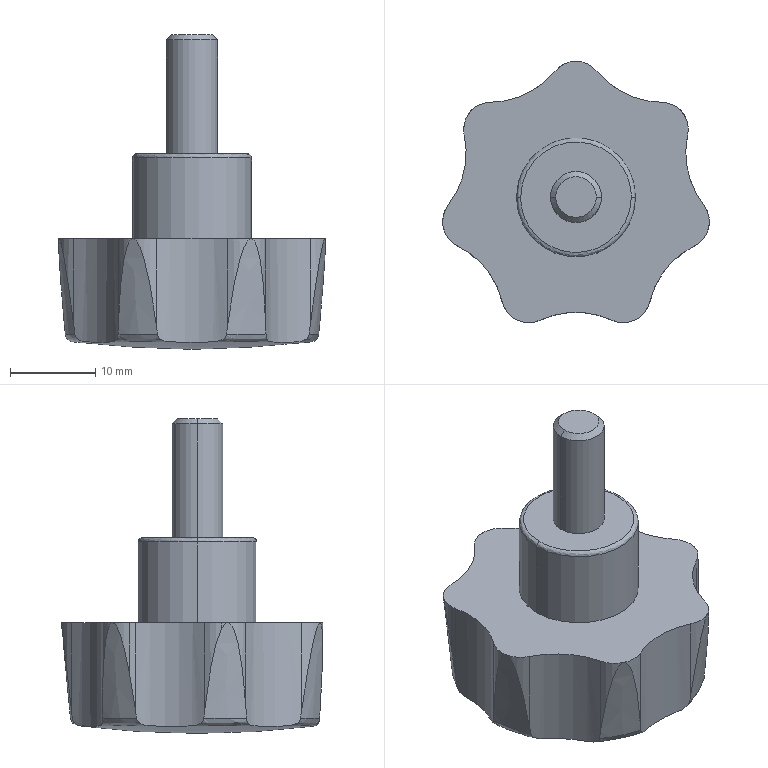Part | SolidWorks | features BaseBody 1 | 1 solid | 50 faces | box 31.358 x 30.732 x 37 mm | volume 10202 mm3 | cylinder 28 | spline 9 | cone 9 | plane 3 | sphere 1 | commonest cylinder face diameters 6.4 x16 20 x8 6 x2 14 x2